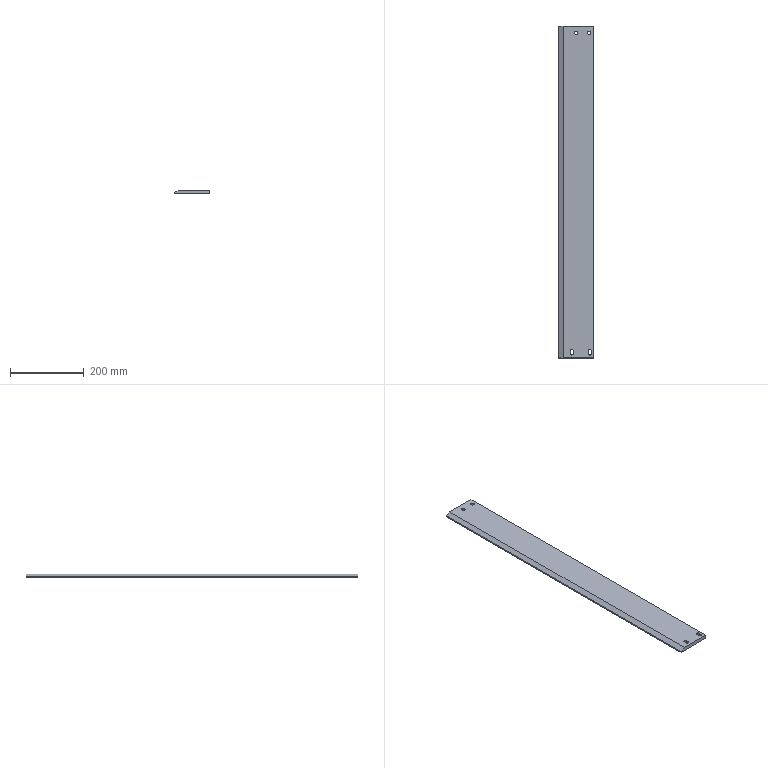Part | NX | features 22 2 | 1 solid | 17 faces | box 95 x 901 x 10 mm | volume 814258 mm3 | plane 11 | cylinder 6 | commonest cylinder face diameters 9 x6
STEP:
#1=CARTESIAN_POINT('',(-124.499,432.45,-13.5));
#2=VERTEX_POINT('',#1);
#3=CARTESIAN_POINT('',(-119.999,432.45,-13.5));
#4=DIRECTION('',(0.,0.,1.));
#5=DIRECTION('',(-1.,0.,0.));
#6=AXIS2_PLACEMENT_3D('',#3,#4,#5);
#7=CIRCLE('',#6,4.5);
#8=EDGE_CURVE('',#2,#2,#7,.T.);
#9=ORIENTED_EDGE('',*,*,#8,.T.);
#10=EDGE_LOOP('',(#9));
#11=FACE_BOUND('',#10,.T.);
#12=CARTESIAN_POINT('',(-89.499,432.45,-13.5));
#13=VERTEX_POINT('',#12);
#14=CARTESIAN_POINT('',(-84.999,432.45,-13.5));
#15=DIRECTION('',(0.,0.,1.));
#16=DIRECTION('',(-1.,0.,0.));
#17=AXIS2_PLACEMENT_3D('',#14,#15,#16);
#18=CIRCLE('',#17,4.5);
#19=EDGE_CURVE('',#13,#13,#18,.T.);
#20=ORIENTED_EDGE('',*,*,#19,.T.);
#21=EDGE_LOOP('',(#20));
#22=FACE_BOUND('',#21,.T.);
#23=CARTESIAN_POINT('',(-73.,450.5,-13.5));
#24=VERTEX_POINT('',#23);
#25=CARTESIAN_POINT('',(-73.,-450.5,-13.5));
#26=VERTEX_POINT('',#25);
#27=CARTESIAN_POINT('',(-73.,468.,-13.5));
#28=DIRECTION('',(0.,-1.,0.));
#29=VECTOR('',#28,1000.);
#30=LINE('',#27,#29);
#31=EDGE_CURVE('',#24,#26,#30,.T.);
#32=ORIENTED_EDGE('',*,*,#31,.T.);
#33=CARTESIAN_POINT('',(-168.,-450.5,-13.5));
#34=VERTEX_POINT('',#33);
#35=CARTESIAN_POINT('',(-58.5,-450.5,-13.5));
#36=DIRECTION('',(-1.,0.,0.));
#37=VECTOR('',#36,1000.);
#38=LINE('',#35,#37);
#39=EDGE_CURVE('',#26,#34,#38,.T.);
#40=ORIENTED_EDGE('',*,*,#39,.T.);
#41=CARTESIAN_POINT('',(-168.,450.5,-13.5));
#42=VERTEX_POINT('',#41);
#43=CARTESIAN_POINT('',(-168.,468.,-13.5));
#44=DIRECTION('',(0.,1.,0.));
#45=VECTOR('',#44,1000.);
#46=LINE('',#43,#45);
#47=EDGE_CURVE('',#34,#42,#46,.T.);
#48=ORIENTED_EDGE('',*,*,#47,.T.);
#49=CARTESIAN_POINT('',(-104.999,450.5,-13.5));
#50=DIRECTION('',(1.,0.,0.));
#51=VECTOR('',#50,1000.);
#52=LINE('',#49,#51);
#53=EDGE_CURVE('',#42,#24,#52,.T.);
#54=ORIENTED_EDGE('',*,*,#53,.T.);
#55=EDGE_LOOP('',(#32,#40,#48,#54));
#56=FACE_BOUND('',#55,.T.);
#57=CARTESIAN_POINT('',(-127.498,-432.,-13.5));
#58=VERTEX_POINT('',#57);
#59=CARTESIAN_POINT('',(-136.498,-432.,-13.5));
#60=VERTEX_POINT('',#59);
#61=CARTESIAN_POINT('',(-131.998,-432.,-13.5));
#62=DIRECTION('',(0.,0.,1.));
#63=DIRECTION('',(-1.,0.,0.));
#64=AXIS2_PLACEMENT_3D('',#61,#62,#63);
#65=CIRCLE('',#64,4.5);
#66=EDGE_CURVE('',#58,#60,#65,.T.);
#67=ORIENTED_EDGE('',*,*,#66,.T.);
#68=CARTESIAN_POINT('',(-136.498,-438.,-13.5));
#69=VERTEX_POINT('',#68);
#70=CARTESIAN_POINT('',(-136.498,-435.,-13.5));
#71=DIRECTION('',(0.,-1.,0.));
#72=VECTOR('',#71,1000.);
#73=LINE('',#70,#72);
#74=EDGE_CURVE('',#60,#69,#73,.T.);
#75=ORIENTED_EDGE('',*,*,#74,.T.);
#76=CARTESIAN_POINT('',(-127.498,-438.,-13.5));
#77=VERTEX_POINT('',#76);
#78=CARTESIAN_POINT('',(-131.998,-438.,-13.5));
#79=DIRECTION('',(0.,0.,1.));
#80=DIRECTION('',(-1.,0.,0.));
#81=AXIS2_PLACEMENT_3D('',#78,#79,#80);
#82=CIRCLE('',#81,4.5);
#83=EDGE_CURVE('',#69,#77,#82,.T.);
#84=ORIENTED_EDGE('',*,*,#83,.T.);
#85=CARTESIAN_POINT('',(-127.498,-435.,-13.5));
#86=DIRECTION('',(0.,1.,0.));
#87=VECTOR('',#86,1000.);
#88=LINE('',#85,#87);
#89=EDGE_CURVE('',#77,#58,#88,.T.);
#90=ORIENTED_EDGE('',*,*,#89,.T.);
#91=EDGE_LOOP('',(#67,#75,#84,#90));
#92=FACE_BOUND('',#91,.T.);
#93=CARTESIAN_POINT('',(-78.498,-438.,-13.5));
#94=VERTEX_POINT('',#93);
#95=CARTESIAN_POINT('',(-78.498,-432.,-13.5));
#96=VERTEX_POINT('',#95);
#97=CARTESIAN_POINT('',(-78.498,-435.,-13.5));
#98=DIRECTION('',(0.,1.,0.));
#99=VECTOR('',#98,1000.);
#100=LINE('',#97,#99);
#101=EDGE_CURVE('',#94,#96,#100,.T.);
#102=ORIENTED_EDGE('',*,*,#101,.T.);
#103=CARTESIAN_POINT('',(-87.498,-432.,-13.5));
#104=VERTEX_POINT('',#103);
#105=CARTESIAN_POINT('',(-82.998,-432.,-13.5));
#106=DIRECTION('',(0.,0.,1.));
#107=DIRECTION('',(-1.,0.,0.));
#108=AXIS2_PLACEMENT_3D('',#105,#106,#107);
#109=CIRCLE('',#108,4.5);
#110=EDGE_CURVE('',#96,#104,#109,.T.);
#111=ORIENTED_EDGE('',*,*,#110,.T.);
#112=CARTESIAN_POINT('',(-87.498,-438.,-13.5));
#113=VERTEX_POINT('',#112);
#114=CARTESIAN_POINT('',(-87.498,-435.,-13.5));
#115=DIRECTION('',(0.,-1.,0.));
#116=VECTOR('',#115,1000.);
#117=LINE('',#114,#116);
#118=EDGE_CURVE('',#104,#113,#117,.T.);
#119=ORIENTED_EDGE('',*,*,#118,.T.);
#120=CARTESIAN_POINT('',(-82.998,-438.,-13.5));
#121=DIRECTION('',(0.,0.,1.));
#122=DIRECTION('',(-1.,0.,0.));
#123=AXIS2_PLACEMENT_3D('',#120,#121,#122);
#124=CIRCLE('',#123,4.5);
#125=EDGE_CURVE('',#113,#94,#124,.T.);
#126=ORIENTED_EDGE('',*,*,#125,.T.);
#127=EDGE_LOOP('',(#102,#111,#119,#126));
#128=FACE_BOUND('',#127,.T.);
#129=CARTESIAN_POINT('',(-58.5,468.,-13.5));
#130=DIRECTION('',(0.,0.,-1.));
#131=DIRECTION('',(-1.,0.,0.));
#132=AXIS2_PLACEMENT_3D('',#129,#130,#131);
#133=PLANE('',#132);
#134=ADVANCED_FACE('',(#11,#22,#56,#92,#128),#133,.T.);
#135=CARTESIAN_POINT('',(-168.,-450.5,-10.));
#136=VERTEX_POINT('',#135);
#137=CARTESIAN_POINT('',(-168.,-450.5,11.));
#138=DIRECTION('',(0.,0.,1.));
#139=VECTOR('',#138,1000.);
#140=LINE('',#137,#139);
#141=EDGE_CURVE('',#34,#136,#140,.T.);
#142=ORIENTED_EDGE('',*,*,#141,.T.);
#143=CARTESIAN_POINT('',(-168.,450.5,-10.));
#144=VERTEX_POINT('',#143);
#145=CARTESIAN_POINT('',(-168.,468.,-10.));
#146=DIRECTION('',(0.,1.,0.));
#147=VECTOR('',#146,1000.);
#148=LINE('',#145,#147);
#149=EDGE_CURVE('',#136,#144,#148,.T.);
#150=ORIENTED_EDGE('',*,*,#149,.T.);
#151=CARTESIAN_POINT('',(-168.,450.5,-3.5));
#152=DIRECTION('',(0.,0.,-1.));
#153=VECTOR('',#152,1000.);
#154=LINE('',#151,#153);
#155=EDGE_CURVE('',#144,#42,#154,.T.);
#156=ORIENTED_EDGE('',*,*,#155,.T.);
#157=ORIENTED_EDGE('',*,*,#47,.F.);
#158=EDGE_LOOP('',(#142,#150,#156,#157));
#159=FACE_BOUND('',#158,.T.);
#160=CARTESIAN_POINT('',(-168.,468.,-3.5));
#161=DIRECTION('',(1.,0.,0.));
#162=DIRECTION('',(0.,-1.,0.));
#163=AXIS2_PLACEMENT_3D('',#160,#161,#162);
#164=PLANE('',#163);
#165=ADVANCED_FACE('',(#159),#164,.F.);
#166=ORIENTED_EDGE('',*,*,#19,.F.);
#167=EDGE_LOOP('',(#166));
#168=FACE_BOUND('',#167,.T.);
#169=CARTESIAN_POINT('',(-89.499,432.45,-3.5));
#170=VERTEX_POINT('',#169);
#171=CARTESIAN_POINT('',(-84.999,432.45,-3.5));
#172=DIRECTION('',(0.,0.,1.));
#173=DIRECTION('',(-1.,0.,0.));
#174=AXIS2_PLACEMENT_3D('',#171,#172,#173);
#175=CIRCLE('',#174,4.5);
#176=EDGE_CURVE('',#170,#170,#175,.T.);
#177=ORIENTED_EDGE('',*,*,#176,.T.);
#178=EDGE_LOOP('',(#177));
#179=FACE_BOUND('',#178,.T.);
#180=CARTESIAN_POINT('',(-84.999,432.45,26.5));
#181=DIRECTION('',(0.,0.,-1.));
#182=DIRECTION('',(-1.,0.,0.));
#183=AXIS2_PLACEMENT_3D('',#180,#181,#182);
#184=CYLINDRICAL_SURFACE('',#183,4.5);
#185=ADVANCED_FACE('',(#168,#179),#184,.F.);
#186=ORIENTED_EDGE('',*,*,#8,.F.);
#187=EDGE_LOOP('',(#186));
#188=FACE_BOUND('',#187,.T.);
#189=CARTESIAN_POINT('',(-124.499,432.45,-3.5));
#190=VERTEX_POINT('',#189);
#191=CARTESIAN_POINT('',(-119.999,432.45,-3.5));
#192=DIRECTION('',(0.,0.,1.));
#193=DIRECTION('',(-1.,0.,0.));
#194=AXIS2_PLACEMENT_3D('',#191,#192,#193);
#195=CIRCLE('',#194,4.5);
#196=EDGE_CURVE('',#190,#190,#195,.T.);
#197=ORIENTED_EDGE('',*,*,#196,.T.);
#198=EDGE_LOOP('',(#197));
#199=FACE_BOUND('',#198,.T.);
#200=CARTESIAN_POINT('',(-119.999,432.45,26.5));
#201=DIRECTION('',(0.,0.,-1.));
#202=DIRECTION('',(-1.,0.,0.));
#203=AXIS2_PLACEMENT_3D('',#200,#201,#202);
#204=CYLINDRICAL_SURFACE('',#203,4.5);
#205=ADVANCED_FACE('',(#188,#199),#204,.F.);
#206=CARTESIAN_POINT('',(-155.,-450.5,-3.5));
#207=VERTEX_POINT('',#206);
#208=CARTESIAN_POINT('',(-165.,-450.5,-8.5));
#209=DIRECTION('',(-0.8944,0.,-0.4472));
#210=VECTOR('',#209,1000.);
#211=LINE('',#208,#210);
#212=EDGE_CURVE('',#207,#136,#211,.T.);
#213=ORIENTED_EDGE('',*,*,#212,.F.);
#214=CARTESIAN_POINT('',(-155.,450.5,-3.5));
#215=VERTEX_POINT('',#214);
#216=CARTESIAN_POINT('',(-155.,-42.,-3.5));
#217=DIRECTION('',(0.,-1.,0.));
#218=VECTOR('',#217,1000.);
#219=LINE('',#216,#218);
#220=EDGE_CURVE('',#215,#207,#219,.T.);
#221=ORIENTED_EDGE('',*,*,#220,.F.);
#222=CARTESIAN_POINT('',(-109.199,450.5,19.4));
#223=DIRECTION('',(0.8944,0.,0.4472));
#224=VECTOR('',#223,1000.);
#225=LINE('',#222,#224);
#226=EDGE_CURVE('',#144,#215,#225,.T.);
#227=ORIENTED_EDGE('',*,*,#226,.F.);
#228=ORIENTED_EDGE('',*,*,#149,.F.);
#229=EDGE_LOOP('',(#213,#221,#227,#228));
#230=FACE_BOUND('',#229,.T.);
#231=CARTESIAN_POINT('',(-165.,468.,-8.5));
#232=DIRECTION('',(0.4472,0.,-0.8944));
#233=DIRECTION('',(0.,1.,0.));
#234=AXIS2_PLACEMENT_3D('',#231,#232,#233);
#235=PLANE('',#234);
#236=ADVANCED_FACE('',(#230),#235,.F.);
#237=CARTESIAN_POINT('',(-73.,450.5,-3.5));
#238=VERTEX_POINT('',#237);
#239=CARTESIAN_POINT('',(-104.999,450.5,-3.5));
#240=DIRECTION('',(1.,0.,0.));
#241=VECTOR('',#240,1000.);
#242=LINE('',#239,#241);
#243=EDGE_CURVE('',#215,#238,#242,.T.);
#244=ORIENTED_EDGE('',*,*,#243,.T.);
#245=CARTESIAN_POINT('',(-73.,450.5,-11.));
#246=DIRECTION('',(0.,0.,-1.));
#247=VECTOR('',#246,1000.);
#248=LINE('',#245,#247);
#249=EDGE_CURVE('',#238,#24,#248,.T.);
#250=ORIENTED_EDGE('',*,*,#249,.T.);
#251=ORIENTED_EDGE('',*,*,#53,.F.);
#252=ORIENTED_EDGE('',*,*,#155,.F.);
#253=ORIENTED_EDGE('',*,*,#226,.T.);
#254=EDGE_LOOP('',(#244,#250,#251,#252,#253));
#255=FACE_BOUND('',#254,.T.);
#256=CARTESIAN_POINT('',(-104.999,450.5,11.));
#257=DIRECTION('',(0.,-1.,0.));
#258=DIRECTION('',(0.,0.,-1.));
#259=AXIS2_PLACEMENT_3D('',#256,#257,#258);
#260=PLANE('',#259);
#261=ADVANCED_FACE('',(#255),#260,.F.);
#262=CARTESIAN_POINT('',(-73.,-450.5,-3.5));
#263=VERTEX_POINT('',#262);
#264=CARTESIAN_POINT('',(-73.,468.,-3.5));
#265=DIRECTION('',(0.,-1.,0.));
#266=VECTOR('',#265,1000.);
#267=LINE('',#264,#266);
#268=EDGE_CURVE('',#238,#263,#267,.T.);
#269=ORIENTED_EDGE('',*,*,#268,.T.);
#270=CARTESIAN_POINT('',(-73.,-450.5,11.));
#271=DIRECTION('',(0.,0.,1.));
#272=VECTOR('',#271,1000.);
#273=LINE('',#270,#272);
#274=EDGE_CURVE('',#26,#263,#273,.T.);
#275=ORIENTED_EDGE('',*,*,#274,.F.);
#276=ORIENTED_EDGE('',*,*,#31,.F.);
#277=ORIENTED_EDGE('',*,*,#249,.F.);
#278=EDGE_LOOP('',(#269,#275,#276,#277));
#279=FACE_BOUND('',#278,.T.);
#280=CARTESIAN_POINT('',(-73.,193.,-11.));
#281=DIRECTION('',(1.,0.,0.));
#282=DIRECTION('',(0.,0.,-1.));
#283=AXIS2_PLACEMENT_3D('',#280,#281,#282);
#284=PLANE('',#283);
#285=ADVANCED_FACE('',(#279),#284,.T.);
#286=ORIENTED_EDGE('',*,*,#39,.F.);
#287=ORIENTED_EDGE('',*,*,#274,.T.);
#288=CARTESIAN_POINT('',(-58.5,-450.5,-3.5));
#289=DIRECTION('',(-1.,0.,0.));
#290=VECTOR('',#289,1000.);
#291=LINE('',#288,#290);
#292=EDGE_CURVE('',#263,#207,#291,.T.);
#293=ORIENTED_EDGE('',*,*,#292,.T.);
#294=ORIENTED_EDGE('',*,*,#212,.T.);
#295=ORIENTED_EDGE('',*,*,#141,.F.);
#296=EDGE_LOOP('',(#286,#287,#293,#294,#295));
#297=FACE_BOUND('',#296,.T.);
#298=CARTESIAN_POINT('',(-125.998,-450.5,11.));
#299=DIRECTION('',(0.,1.,0.));
#300=DIRECTION('',(0.,0.,-1.));
#301=AXIS2_PLACEMENT_3D('',#298,#299,#300);
#302=PLANE('',#301);
#303=ADVANCED_FACE('',(#297),#302,.F.);
#304=ORIENTED_EDGE('',*,*,#292,.F.);
#305=ORIENTED_EDGE('',*,*,#268,.F.);
#306=ORIENTED_EDGE('',*,*,#243,.F.);
#307=ORIENTED_EDGE('',*,*,#220,.T.);
#308=EDGE_LOOP('',(#304,#305,#306,#307));
#309=FACE_BOUND('',#308,.T.);
#310=ORIENTED_EDGE('',*,*,#196,.F.);
#311=EDGE_LOOP('',(#310));
#312=FACE_BOUND('',#311,.T.);
#313=CARTESIAN_POINT('',(-136.498,-438.,-3.5));
#314=VERTEX_POINT('',#313);
#315=CARTESIAN_POINT('',(-136.498,-432.,-3.5));
#316=VERTEX_POINT('',#315);
#317=CARTESIAN_POINT('',(-136.498,-435.,-3.5));
#318=DIRECTION('',(0.,1.,0.));
#319=VECTOR('',#318,1000.);
#320=LINE('',#317,#319);
#321=EDGE_CURVE('',#314,#316,#320,.T.);
#322=ORIENTED_EDGE('',*,*,#321,.T.);
#323=CARTESIAN_POINT('',(-127.498,-432.,-3.5));
#324=VERTEX_POINT('',#323);
#325=CARTESIAN_POINT('',(-131.998,-432.,-3.5));
#326=DIRECTION('',(0.,0.,-1.));
#327=DIRECTION('',(-1.,0.,0.));
#328=AXIS2_PLACEMENT_3D('',#325,#326,#327);
#329=CIRCLE('',#328,4.5);
#330=EDGE_CURVE('',#316,#324,#329,.T.);
#331=ORIENTED_EDGE('',*,*,#330,.T.);
#332=CARTESIAN_POINT('',(-127.498,-438.,-3.5));
#333=VERTEX_POINT('',#332);
#334=CARTESIAN_POINT('',(-127.498,-435.,-3.5));
#335=DIRECTION('',(0.,-1.,0.));
#336=VECTOR('',#335,1000.);
#337=LINE('',#334,#336);
#338=EDGE_CURVE('',#324,#333,#337,.T.);
#339=ORIENTED_EDGE('',*,*,#338,.T.);
#340=CARTESIAN_POINT('',(-131.998,-438.,-3.5));
#341=DIRECTION('',(0.,0.,-1.));
#342=DIRECTION('',(-1.,0.,0.));
#343=AXIS2_PLACEMENT_3D('',#340,#341,#342);
#344=CIRCLE('',#343,4.5);
#345=EDGE_CURVE('',#333,#314,#344,.T.);
#346=ORIENTED_EDGE('',*,*,#345,.T.);
#347=EDGE_LOOP('',(#322,#331,#339,#346));
#348=FACE_BOUND('',#347,.T.);
#349=ORIENTED_EDGE('',*,*,#176,.F.);
#350=EDGE_LOOP('',(#349));
#351=FACE_BOUND('',#350,.T.);
#352=CARTESIAN_POINT('',(-87.498,-432.,-3.5));
#353=VERTEX_POINT('',#352);
#354=CARTESIAN_POINT('',(-78.498,-432.,-3.5));
#355=VERTEX_POINT('',#354);
#356=CARTESIAN_POINT('',(-82.998,-432.,-3.5));
#357=DIRECTION('',(0.,0.,-1.));
#358=DIRECTION('',(-1.,0.,0.));
#359=AXIS2_PLACEMENT_3D('',#356,#357,#358);
#360=CIRCLE('',#359,4.5);
#361=EDGE_CURVE('',#353,#355,#360,.T.);
#362=ORIENTED_EDGE('',*,*,#361,.T.);
#363=CARTESIAN_POINT('',(-78.498,-438.,-3.5));
#364=VERTEX_POINT('',#363);
#365=CARTESIAN_POINT('',(-78.498,-435.,-3.5));
#366=DIRECTION('',(0.,-1.,0.));
#367=VECTOR('',#366,1000.);
#368=LINE('',#365,#367);
#369=EDGE_CURVE('',#355,#364,#368,.T.);
#370=ORIENTED_EDGE('',*,*,#369,.T.);
#371=CARTESIAN_POINT('',(-87.498,-438.,-3.5));
#372=VERTEX_POINT('',#371);
#373=CARTESIAN_POINT('',(-82.998,-438.,-3.5));
#374=DIRECTION('',(0.,0.,-1.));
#375=DIRECTION('',(-1.,0.,0.));
#376=AXIS2_PLACEMENT_3D('',#373,#374,#375);
#377=CIRCLE('',#376,4.5);
#378=EDGE_CURVE('',#364,#372,#377,.T.);
#379=ORIENTED_EDGE('',*,*,#378,.T.);
#380=CARTESIAN_POINT('',(-87.498,-435.,-3.5));
#381=DIRECTION('',(0.,1.,0.));
#382=VECTOR('',#381,1000.);
#383=LINE('',#380,#382);
#384=EDGE_CURVE('',#372,#353,#383,.T.);
#385=ORIENTED_EDGE('',*,*,#384,.T.);
#386=EDGE_LOOP('',(#362,#370,#379,#385));
#387=FACE_BOUND('',#386,.T.);
#388=CARTESIAN_POINT('',(-58.5,468.,-3.5));
#389=DIRECTION('',(0.,0.,-1.));
#390=DIRECTION('',(-1.,0.,0.));
#391=AXIS2_PLACEMENT_3D('',#388,#389,#390);
#392=PLANE('',#391);
#393=ADVANCED_FACE('',(#309,#312,#348,#351,#387),#392,.F.);
#394=ORIENTED_EDGE('',*,*,#74,.F.);
#395=CARTESIAN_POINT('',(-136.498,-432.,-3.5));
#396=DIRECTION('',(0.,0.,1.));
#397=VECTOR('',#396,1000.);
#398=LINE('',#395,#397);
#399=EDGE_CURVE('',#60,#316,#398,.T.);
#400=ORIENTED_EDGE('',*,*,#399,.T.);
#401=ORIENTED_EDGE('',*,*,#321,.F.);
#402=CARTESIAN_POINT('',(-136.498,-438.,-13.5));
#403=DIRECTION('',(0.,0.,-1.));
#404=VECTOR('',#403,1000.);
#405=LINE('',#402,#404);
#406=EDGE_CURVE('',#314,#69,#405,.T.);
#407=ORIENTED_EDGE('',*,*,#406,.T.);
#408=EDGE_LOOP('',(#394,#400,#401,#407));
#409=FACE_BOUND('',#408,.T.);
#410=CARTESIAN_POINT('',(-136.498,-435.,-13.5));
#411=DIRECTION('',(-1.,0.,0.));
#412=DIRECTION('',(0.,0.,1.));
#413=AXIS2_PLACEMENT_3D('',#410,#411,#412);
#414=PLANE('',#413);
#415=ADVANCED_FACE('',(#409),#414,.F.);
#416=ORIENTED_EDGE('',*,*,#338,.F.);
#417=CARTESIAN_POINT('',(-127.498,-432.,-13.5));
#418=DIRECTION('',(0.,0.,-1.));
#419=VECTOR('',#418,1000.);
#420=LINE('',#417,#419);
#421=EDGE_CURVE('',#324,#58,#420,.T.);
#422=ORIENTED_EDGE('',*,*,#421,.T.);
#423=ORIENTED_EDGE('',*,*,#89,.F.);
#424=CARTESIAN_POINT('',(-127.498,-438.,-3.5));
#425=DIRECTION('',(0.,0.,1.));
#426=VECTOR('',#425,1000.);
#427=LINE('',#424,#426);
#428=EDGE_CURVE('',#77,#333,#427,.T.);
#429=ORIENTED_EDGE('',*,*,#428,.T.);
#430=EDGE_LOOP('',(#416,#422,#423,#429));
#431=FACE_BOUND('',#430,.T.);
#432=CARTESIAN_POINT('',(-127.498,-435.,-13.5));
#433=DIRECTION('',(1.,0.,0.));
#434=DIRECTION('',(0.,0.,-1.));
#435=AXIS2_PLACEMENT_3D('',#432,#433,#434);
#436=PLANE('',#435);
#437=ADVANCED_FACE('',(#431),#436,.F.);
#438=ORIENTED_EDGE('',*,*,#118,.F.);
#439=CARTESIAN_POINT('',(-87.498,-432.,-3.5));
#440=DIRECTION('',(0.,0.,1.));
#441=VECTOR('',#440,1000.);
#442=LINE('',#439,#441);
#443=EDGE_CURVE('',#104,#353,#442,.T.);
#444=ORIENTED_EDGE('',*,*,#443,.T.);
#445=ORIENTED_EDGE('',*,*,#384,.F.);
#446=CARTESIAN_POINT('',(-87.498,-438.,-13.5));
#447=DIRECTION('',(0.,0.,-1.));
#448=VECTOR('',#447,1000.);
#449=LINE('',#446,#448);
#450=EDGE_CURVE('',#372,#113,#449,.T.);
#451=ORIENTED_EDGE('',*,*,#450,.T.);
#452=EDGE_LOOP('',(#438,#444,#445,#451));
#453=FACE_BOUND('',#452,.T.);
#454=CARTESIAN_POINT('',(-87.498,-435.,-13.5));
#455=DIRECTION('',(-1.,0.,0.));
#456=DIRECTION('',(0.,0.,1.));
#457=AXIS2_PLACEMENT_3D('',#454,#455,#456);
#458=PLANE('',#457);
#459=ADVANCED_FACE('',(#453),#458,.F.);
#460=ORIENTED_EDGE('',*,*,#369,.F.);
#461=CARTESIAN_POINT('',(-78.498,-432.,-13.5));
#462=DIRECTION('',(0.,0.,-1.));
#463=VECTOR('',#462,1000.);
#464=LINE('',#461,#463);
#465=EDGE_CURVE('',#355,#96,#464,.T.);
#466=ORIENTED_EDGE('',*,*,#465,.T.);
#467=ORIENTED_EDGE('',*,*,#101,.F.);
#468=CARTESIAN_POINT('',(-78.498,-438.,-3.5));
#469=DIRECTION('',(0.,0.,1.));
#470=VECTOR('',#469,1000.);
#471=LINE('',#468,#470);
#472=EDGE_CURVE('',#94,#364,#471,.T.);
#473=ORIENTED_EDGE('',*,*,#472,.T.);
#474=EDGE_LOOP('',(#460,#466,#467,#473));
#475=FACE_BOUND('',#474,.T.);
#476=CARTESIAN_POINT('',(-78.498,-435.,-13.5));
#477=DIRECTION('',(1.,0.,0.));
#478=DIRECTION('',(0.,0.,-1.));
#479=AXIS2_PLACEMENT_3D('',#476,#477,#478);
#480=PLANE('',#479);
#481=ADVANCED_FACE('',(#475),#480,.F.);
#482=ORIENTED_EDGE('',*,*,#399,.F.);
#483=ORIENTED_EDGE('',*,*,#66,.F.);
#484=ORIENTED_EDGE('',*,*,#421,.F.);
#485=ORIENTED_EDGE('',*,*,#330,.F.);
#486=EDGE_LOOP('',(#482,#483,#484,#485));
#487=FACE_BOUND('',#486,.T.);
#488=CARTESIAN_POINT('',(-131.998,-432.,-13.5));
#489=DIRECTION('',(0.,0.,1.));
#490=DIRECTION('',(1.,0.,0.));
#491=AXIS2_PLACEMENT_3D('',#488,#489,#490);
#492=CYLINDRICAL_SURFACE('',#491,4.5);
#493=ADVANCED_FACE('',(#487),#492,.F.);
#494=ORIENTED_EDGE('',*,*,#465,.F.);
#495=ORIENTED_EDGE('',*,*,#361,.F.);
#496=ORIENTED_EDGE('',*,*,#443,.F.);
#497=ORIENTED_EDGE('',*,*,#110,.F.);
#498=EDGE_LOOP('',(#494,#495,#496,#497));
#499=FACE_BOUND('',#498,.T.);
#500=CARTESIAN_POINT('',(-82.998,-432.,-13.5));
#501=DIRECTION('',(0.,0.,1.));
#502=DIRECTION('',(1.,0.,0.));
#503=AXIS2_PLACEMENT_3D('',#500,#501,#502);
#504=CYLINDRICAL_SURFACE('',#503,4.5);
#505=ADVANCED_FACE('',(#499),#504,.F.);
#506=ORIENTED_EDGE('',*,*,#472,.F.);
#507=ORIENTED_EDGE('',*,*,#125,.F.);
#508=ORIENTED_EDGE('',*,*,#450,.F.);
#509=ORIENTED_EDGE('',*,*,#378,.F.);
#510=EDGE_LOOP('',(#506,#507,#508,#509));
#511=FACE_BOUND('',#510,.T.);
#512=CARTESIAN_POINT('',(-82.998,-438.,-13.5));
#513=DIRECTION('',(0.,0.,1.));
#514=DIRECTION('',(1.,0.,0.));
#515=AXIS2_PLACEMENT_3D('',#512,#513,#514);
#516=CYLINDRICAL_SURFACE('',#515,4.5);
#517=ADVANCED_FACE('',(#511),#516,.F.);
#518=ORIENTED_EDGE('',*,*,#406,.F.);
#519=ORIENTED_EDGE('',*,*,#345,.F.);
#520=ORIENTED_EDGE('',*,*,#428,.F.);
#521=ORIENTED_EDGE('',*,*,#83,.F.);
#522=EDGE_LOOP('',(#518,#519,#520,#521));
#523=FACE_BOUND('',#522,.T.);
#524=CARTESIAN_POINT('',(-131.998,-438.,-13.5));
#525=DIRECTION('',(0.,0.,1.));
#526=DIRECTION('',(1.,0.,0.));
#527=AXIS2_PLACEMENT_3D('',#524,#525,#526);
#528=CYLINDRICAL_SURFACE('',#527,4.5);
#529=ADVANCED_FACE('',(#523),#528,.F.);
#530=CLOSED_SHELL('',(#134,#165,#185,#205,#236,#261,#285,#303,#393,#415,#437,#459,#481,#493,#505,#517,#529));
#531=MANIFOLD_SOLID_BREP('',#530);
#532=(LENGTH_UNIT()NAMED_UNIT(*)SI_UNIT(.MILLI.,.METRE.));
#533=UNCERTAINTY_MEASURE_WITH_UNIT(LENGTH_MEASURE(0.00001),#532,'','');
#534=(NAMED_UNIT(*)PLANE_ANGLE_UNIT()SI_UNIT($,.RADIAN.));
#535=(NAMED_UNIT(*)SI_UNIT($,.STERADIAN.)SOLID_ANGLE_UNIT());
#536=(GEOMETRIC_REPRESENTATION_CONTEXT(3)GLOBAL_UNCERTAINTY_ASSIGNED_CONTEXT((#533))GLOBAL_UNIT_ASSIGNED_CONTEXT((#532,#534,#535))REPRESENTATION_CONTEXT('',''));
#537=ADVANCED_BREP_SHAPE_REPRESENTATION('',(#531),#536);